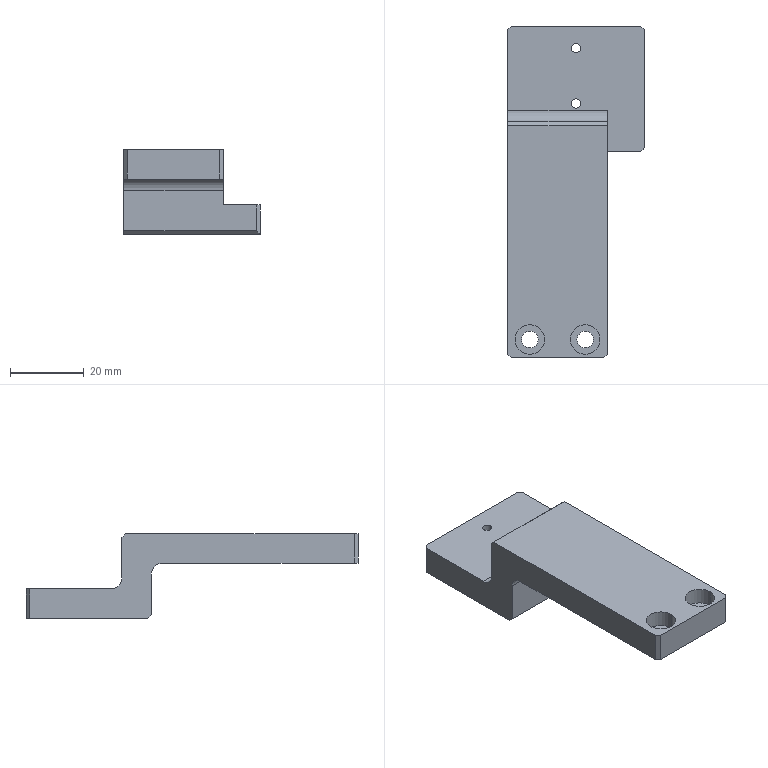Part | SolidWorks | features ICE 3, Chamfer 2, HoleWzd 2, Extrusion 1, Fillet 1 | 1 solid | 34 faces | box 37 x 90 x 23 mm | volume 24810 mm3 | plane 20 | cylinder 14 | commonest cylinder face diameters 2.5 x4 4.5 x4 8 x4 6 x2
STEP:
#1=CARTESIAN_POINT('',(2.,-85.,-0.5));
#2=VERTEX_POINT('',#1);
#3=CARTESIAN_POINT('',(10.,-85.,-0.5));
#4=VERTEX_POINT('',#3);
#5=CARTESIAN_POINT('',(6.,-85.,-0.5));
#6=DIRECTION('',(0.,0.,1.));
#7=DIRECTION('',(1.,0.,0.));
#8=AXIS2_PLACEMENT_3D('',#5,#6,#7);
#9=CIRCLE('',#8,4.);
#10=EDGE_CURVE('',#2,#4,#9,.T.);
#11=ORIENTED_EDGE('',*,*,#10,.F.);
#12=CARTESIAN_POINT('',(2.,-85.,4.));
#13=VERTEX_POINT('',#12);
#14=CARTESIAN_POINT('',(2.,-85.,4.));
#15=DIRECTION('',(0.,0.,1.));
#16=VECTOR('',#15,1000.);
#17=LINE('',#14,#16);
#18=EDGE_CURVE('',#2,#13,#17,.T.);
#19=ORIENTED_EDGE('',*,*,#18,.T.);
#20=CARTESIAN_POINT('',(10.,-85.,4.));
#21=VERTEX_POINT('',#20);
#22=CARTESIAN_POINT('',(6.,-85.,4.));
#23=DIRECTION('',(0.,0.,1.));
#24=DIRECTION('',(1.,0.,0.));
#25=AXIS2_PLACEMENT_3D('',#22,#23,#24);
#26=CIRCLE('',#25,4.);
#27=EDGE_CURVE('',#13,#21,#26,.T.);
#28=ORIENTED_EDGE('',*,*,#27,.T.);
#29=CARTESIAN_POINT('',(10.,-85.,4.));
#30=DIRECTION('',(0.,0.,1.));
#31=VECTOR('',#30,1000.);
#32=LINE('',#29,#31);
#33=EDGE_CURVE('',#4,#21,#32,.T.);
#34=ORIENTED_EDGE('',*,*,#33,.F.);
#35=EDGE_LOOP('',(#11,#19,#28,#34));
#36=FACE_OUTER_BOUND('',#35,.T.);
#37=CARTESIAN_POINT('',(6.,-85.,4.));
#38=DIRECTION('',(0.,0.,1.));
#39=DIRECTION('',(1.,0.,0.));
#40=AXIS2_PLACEMENT_3D('',#37,#38,#39);
#41=CYLINDRICAL_SURFACE('',#40,4.);
#42=ADVANCED_FACE('',(#36),#41,.F.);
#43=CARTESIAN_POINT('',(3.75,-85.,-4.));
#44=VERTEX_POINT('',#43);
#45=CARTESIAN_POINT('',(8.25,-85.,-4.));
#46=VERTEX_POINT('',#45);
#47=CARTESIAN_POINT('',(6.,-85.,-4.));
#48=DIRECTION('',(0.,0.,1.));
#49=DIRECTION('',(1.,0.,0.));
#50=AXIS2_PLACEMENT_3D('',#47,#48,#49);
#51=CIRCLE('',#50,2.25);
#52=EDGE_CURVE('',#44,#46,#51,.T.);
#53=ORIENTED_EDGE('',*,*,#52,.F.);
#54=CARTESIAN_POINT('',(3.75,-85.,-0.5));
#55=VERTEX_POINT('',#54);
#56=CARTESIAN_POINT('',(3.75,-85.,4.));
#57=DIRECTION('',(0.,0.,1.));
#58=VECTOR('',#57,1000.);
#59=LINE('',#56,#58);
#60=EDGE_CURVE('',#44,#55,#59,.T.);
#61=ORIENTED_EDGE('',*,*,#60,.T.);
#62=CARTESIAN_POINT('',(8.25,-85.,-0.5));
#63=VERTEX_POINT('',#62);
#64=CARTESIAN_POINT('',(6.,-85.,-0.5));
#65=DIRECTION('',(0.,0.,1.));
#66=DIRECTION('',(1.,0.,0.));
#67=AXIS2_PLACEMENT_3D('',#64,#65,#66);
#68=CIRCLE('',#67,2.25);
#69=EDGE_CURVE('',#55,#63,#68,.T.);
#70=ORIENTED_EDGE('',*,*,#69,.T.);
#71=CARTESIAN_POINT('',(8.25,-85.,4.));
#72=DIRECTION('',(0.,0.,1.));
#73=VECTOR('',#72,1000.);
#74=LINE('',#71,#73);
#75=EDGE_CURVE('',#46,#63,#74,.T.);
#76=ORIENTED_EDGE('',*,*,#75,.F.);
#77=EDGE_LOOP('',(#53,#61,#70,#76));
#78=FACE_OUTER_BOUND('',#77,.T.);
#79=CARTESIAN_POINT('',(6.,-85.,4.));
#80=DIRECTION('',(0.,0.,1.));
#81=DIRECTION('',(1.,0.,0.));
#82=AXIS2_PLACEMENT_3D('',#79,#80,#81);
#83=CYLINDRICAL_SURFACE('',#82,2.25);
#84=ADVANCED_FACE('',(#78),#83,.F.);
#85=CARTESIAN_POINT('',(17.,-85.,-0.5));
#86=VERTEX_POINT('',#85);
#87=CARTESIAN_POINT('',(25.,-85.,-0.5));
#88=VERTEX_POINT('',#87);
#89=CARTESIAN_POINT('',(21.,-85.,-0.5));
#90=DIRECTION('',(0.,0.,1.));
#91=DIRECTION('',(1.,0.,0.));
#92=AXIS2_PLACEMENT_3D('',#89,#90,#91);
#93=CIRCLE('',#92,4.);
#94=EDGE_CURVE('',#86,#88,#93,.T.);
#95=ORIENTED_EDGE('',*,*,#94,.F.);
#96=CARTESIAN_POINT('',(17.,-85.,4.));
#97=VERTEX_POINT('',#96);
#98=CARTESIAN_POINT('',(17.,-85.,4.));
#99=DIRECTION('',(0.,0.,1.));
#100=VECTOR('',#99,1000.);
#101=LINE('',#98,#100);
#102=EDGE_CURVE('',#86,#97,#101,.T.);
#103=ORIENTED_EDGE('',*,*,#102,.T.);
#104=CARTESIAN_POINT('',(25.,-85.,4.));
#105=VERTEX_POINT('',#104);
#106=CARTESIAN_POINT('',(21.,-85.,4.));
#107=DIRECTION('',(0.,0.,1.));
#108=DIRECTION('',(1.,0.,0.));
#109=AXIS2_PLACEMENT_3D('',#106,#107,#108);
#110=CIRCLE('',#109,4.);
#111=EDGE_CURVE('',#97,#105,#110,.T.);
#112=ORIENTED_EDGE('',*,*,#111,.T.);
#113=CARTESIAN_POINT('',(25.,-85.,4.));
#114=DIRECTION('',(0.,0.,1.));
#115=VECTOR('',#114,1000.);
#116=LINE('',#113,#115);
#117=EDGE_CURVE('',#88,#105,#116,.T.);
#118=ORIENTED_EDGE('',*,*,#117,.F.);
#119=EDGE_LOOP('',(#95,#103,#112,#118));
#120=FACE_OUTER_BOUND('',#119,.T.);
#121=CARTESIAN_POINT('',(21.,-85.,4.));
#122=DIRECTION('',(0.,0.,1.));
#123=DIRECTION('',(1.,0.,0.));
#124=AXIS2_PLACEMENT_3D('',#121,#122,#123);
#125=CYLINDRICAL_SURFACE('',#124,4.);
#126=ADVANCED_FACE('',(#120),#125,.F.);
#127=CARTESIAN_POINT('',(18.75,-85.,-4.));
#128=VERTEX_POINT('',#127);
#129=CARTESIAN_POINT('',(23.25,-85.,-4.));
#130=VERTEX_POINT('',#129);
#131=CARTESIAN_POINT('',(21.,-85.,-4.));
#132=DIRECTION('',(0.,0.,1.));
#133=DIRECTION('',(1.,0.,0.));
#134=AXIS2_PLACEMENT_3D('',#131,#132,#133);
#135=CIRCLE('',#134,2.25);
#136=EDGE_CURVE('',#128,#130,#135,.T.);
#137=ORIENTED_EDGE('',*,*,#136,.F.);
#138=CARTESIAN_POINT('',(18.75,-85.,-0.5));
#139=VERTEX_POINT('',#138);
#140=CARTESIAN_POINT('',(18.75,-85.,4.));
#141=DIRECTION('',(0.,0.,1.));
#142=VECTOR('',#141,1000.);
#143=LINE('',#140,#142);
#144=EDGE_CURVE('',#128,#139,#143,.T.);
#145=ORIENTED_EDGE('',*,*,#144,.T.);
#146=CARTESIAN_POINT('',(23.25,-85.,-0.5));
#147=VERTEX_POINT('',#146);
#148=CARTESIAN_POINT('',(21.,-85.,-0.5));
#149=DIRECTION('',(0.,0.,1.));
#150=DIRECTION('',(1.,0.,0.));
#151=AXIS2_PLACEMENT_3D('',#148,#149,#150);
#152=CIRCLE('',#151,2.25);
#153=EDGE_CURVE('',#139,#147,#152,.T.);
#154=ORIENTED_EDGE('',*,*,#153,.T.);
#155=CARTESIAN_POINT('',(23.25,-85.,4.));
#156=DIRECTION('',(0.,0.,1.));
#157=VECTOR('',#156,1000.);
#158=LINE('',#155,#157);
#159=EDGE_CURVE('',#130,#147,#158,.T.);
#160=ORIENTED_EDGE('',*,*,#159,.F.);
#161=EDGE_LOOP('',(#137,#145,#154,#160));
#162=FACE_OUTER_BOUND('',#161,.T.);
#163=CARTESIAN_POINT('',(21.,-85.,4.));
#164=DIRECTION('',(0.,0.,1.));
#165=DIRECTION('',(1.,0.,0.));
#166=AXIS2_PLACEMENT_3D('',#163,#164,#165);
#167=CYLINDRICAL_SURFACE('',#166,2.25);
#168=ADVANCED_FACE('',(#162),#167,.F.);
#169=CARTESIAN_POINT('',(17.25,-21.,-19.));
#170=VERTEX_POINT('',#169);
#171=CARTESIAN_POINT('',(19.75,-21.,-19.));
#172=VERTEX_POINT('',#171);
#173=CARTESIAN_POINT('',(18.5,-21.,-19.));
#174=DIRECTION('',(0.,0.,1.));
#175=DIRECTION('',(1.,0.,0.));
#176=AXIS2_PLACEMENT_3D('',#173,#174,#175);
#177=CIRCLE('',#176,1.25);
#178=EDGE_CURVE('',#170,#172,#177,.T.);
#179=ORIENTED_EDGE('',*,*,#178,.F.);
#180=CARTESIAN_POINT('',(17.25,-21.,-11.));
#181=VERTEX_POINT('',#180);
#182=CARTESIAN_POINT('',(17.25,-21.,4.));
#183=DIRECTION('',(0.,0.,1.));
#184=VECTOR('',#183,1000.);
#185=LINE('',#182,#184);
#186=EDGE_CURVE('',#170,#181,#185,.T.);
#187=ORIENTED_EDGE('',*,*,#186,.T.);
#188=CARTESIAN_POINT('',(19.75,-21.,-11.));
#189=VERTEX_POINT('',#188);
#190=CARTESIAN_POINT('',(18.5,-21.,-11.));
#191=DIRECTION('',(0.,0.,1.));
#192=DIRECTION('',(0.,1.,0.));
#193=AXIS2_PLACEMENT_3D('',#190,#191,#192);
#194=CIRCLE('',#193,1.25);
#195=EDGE_CURVE('',#181,#189,#194,.T.);
#196=ORIENTED_EDGE('',*,*,#195,.T.);
#197=CARTESIAN_POINT('',(19.75,-21.,4.));
#198=DIRECTION('',(0.,0.,1.));
#199=VECTOR('',#198,1000.);
#200=LINE('',#197,#199);
#201=EDGE_CURVE('',#172,#189,#200,.T.);
#202=ORIENTED_EDGE('',*,*,#201,.F.);
#203=EDGE_LOOP('',(#179,#187,#196,#202));
#204=FACE_OUTER_BOUND('',#203,.T.);
#205=CARTESIAN_POINT('',(18.5,-21.,4.));
#206=DIRECTION('',(0.,0.,1.));
#207=DIRECTION('',(1.,0.,0.));
#208=AXIS2_PLACEMENT_3D('',#205,#206,#207);
#209=CYLINDRICAL_SURFACE('',#208,1.25);
#210=ADVANCED_FACE('',(#204),#209,.F.);
#211=CARTESIAN_POINT('',(17.25,-6.,-19.));
#212=VERTEX_POINT('',#211);
#213=CARTESIAN_POINT('',(19.75,-6.,-19.));
#214=VERTEX_POINT('',#213);
#215=CARTESIAN_POINT('',(18.5,-6.,-19.));
#216=DIRECTION('',(0.,0.,1.));
#217=DIRECTION('',(1.,0.,0.));
#218=AXIS2_PLACEMENT_3D('',#215,#216,#217);
#219=CIRCLE('',#218,1.25);
#220=EDGE_CURVE('',#212,#214,#219,.T.);
#221=ORIENTED_EDGE('',*,*,#220,.F.);
#222=CARTESIAN_POINT('',(17.25,-6.,-11.));
#223=VERTEX_POINT('',#222);
#224=CARTESIAN_POINT('',(17.25,-6.,4.));
#225=DIRECTION('',(0.,0.,1.));
#226=VECTOR('',#225,1000.);
#227=LINE('',#224,#226);
#228=EDGE_CURVE('',#212,#223,#227,.T.);
#229=ORIENTED_EDGE('',*,*,#228,.T.);
#230=CARTESIAN_POINT('',(19.75,-6.,-11.));
#231=VERTEX_POINT('',#230);
#232=CARTESIAN_POINT('',(18.5,-6.,-11.));
#233=DIRECTION('',(0.,0.,1.));
#234=DIRECTION('',(0.,1.,0.));
#235=AXIS2_PLACEMENT_3D('',#232,#233,#234);
#236=CIRCLE('',#235,1.25);
#237=EDGE_CURVE('',#223,#231,#236,.T.);
#238=ORIENTED_EDGE('',*,*,#237,.T.);
#239=CARTESIAN_POINT('',(19.75,-6.,4.));
#240=DIRECTION('',(0.,0.,1.));
#241=VECTOR('',#240,1000.);
#242=LINE('',#239,#241);
#243=EDGE_CURVE('',#214,#231,#242,.T.);
#244=ORIENTED_EDGE('',*,*,#243,.F.);
#245=EDGE_LOOP('',(#221,#229,#238,#244));
#246=FACE_OUTER_BOUND('',#245,.T.);
#247=CARTESIAN_POINT('',(18.5,-6.,4.));
#248=DIRECTION('',(0.,0.,1.));
#249=DIRECTION('',(1.,0.,0.));
#250=AXIS2_PLACEMENT_3D('',#247,#248,#249);
#251=CYLINDRICAL_SURFACE('',#250,1.25);
#252=ADVANCED_FACE('',(#246),#251,.F.);
#253=CARTESIAN_POINT('',(0.,-1.,-19.));
#254=VERTEX_POINT('',#253);
#255=CARTESIAN_POINT('',(0.,-33.,-19.));
#256=VERTEX_POINT('',#255);
#257=CARTESIAN_POINT('',(0.,0.,-19.));
#258=DIRECTION('',(0.,-1.,0.));
#259=VECTOR('',#258,1000.);
#260=LINE('',#257,#259);
#261=EDGE_CURVE('',#254,#256,#260,.T.);
#262=ORIENTED_EDGE('',*,*,#261,.T.);
#263=CARTESIAN_POINT('',(0.,-34.,-18.));
#264=VERTEX_POINT('',#263);
#265=CARTESIAN_POINT('',(0.,-34.,-18.));
#266=DIRECTION('',(0.,-0.7071,0.7071));
#267=VECTOR('',#266,1000.);
#268=LINE('',#265,#267);
#269=EDGE_CURVE('',#256,#264,#268,.T.);
#270=ORIENTED_EDGE('',*,*,#269,.T.);
#271=CARTESIAN_POINT('',(0.,-34.,-7.));
#272=VERTEX_POINT('',#271);
#273=CARTESIAN_POINT('',(0.,-34.,-19.));
#274=DIRECTION('',(0.,0.,1.));
#275=VECTOR('',#274,1000.);
#276=LINE('',#273,#275);
#277=EDGE_CURVE('',#264,#272,#276,.T.);
#278=ORIENTED_EDGE('',*,*,#277,.T.);
#279=CARTESIAN_POINT('',(0.,-37.,-4.));
#280=VERTEX_POINT('',#279);
#281=CARTESIAN_POINT('',(0.,-37.,-7.));
#282=DIRECTION('',(1.,0.,0.));
#283=DIRECTION('',(0.,1.,0.));
#284=AXIS2_PLACEMENT_3D('',#281,#282,#283);
#285=CIRCLE('',#284,3.);
#286=EDGE_CURVE('',#272,#280,#285,.T.);
#287=ORIENTED_EDGE('',*,*,#286,.T.);
#288=CARTESIAN_POINT('',(0.,-89.,-4.));
#289=VERTEX_POINT('',#288);
#290=CARTESIAN_POINT('',(0.,0.,-4.));
#291=DIRECTION('',(0.,-1.,0.));
#292=VECTOR('',#291,1000.);
#293=LINE('',#290,#292);
#294=EDGE_CURVE('',#280,#289,#293,.T.);
#295=ORIENTED_EDGE('',*,*,#294,.T.);
#296=CARTESIAN_POINT('',(0.,-89.,4.));
#297=VERTEX_POINT('',#296);
#298=CARTESIAN_POINT('',(0.,-89.,4.));
#299=DIRECTION('',(0.,0.,1.));
#300=VECTOR('',#299,1000.);
#301=LINE('',#298,#300);
#302=EDGE_CURVE('',#289,#297,#301,.T.);
#303=ORIENTED_EDGE('',*,*,#302,.T.);
#304=CARTESIAN_POINT('',(0.,-27.,4.));
#305=VERTEX_POINT('',#304);
#306=CARTESIAN_POINT('',(0.,0.,4.));
#307=DIRECTION('',(0.,-1.,0.));
#308=VECTOR('',#307,1000.);
#309=LINE('',#306,#308);
#310=EDGE_CURVE('',#305,#297,#309,.T.);
#311=ORIENTED_EDGE('',*,*,#310,.F.);
#312=CARTESIAN_POINT('',(0.,-26.,3.));
#313=VERTEX_POINT('',#312);
#314=CARTESIAN_POINT('',(0.,-26.,3.));
#315=DIRECTION('',(0.,0.7071,-0.7071));
#316=VECTOR('',#315,1000.);
#317=LINE('',#314,#316);
#318=EDGE_CURVE('',#305,#313,#317,.T.);
#319=ORIENTED_EDGE('',*,*,#318,.T.);
#320=CARTESIAN_POINT('',(0.,-26.,-8.));
#321=VERTEX_POINT('',#320);
#322=CARTESIAN_POINT('',(0.,-26.,4.));
#323=DIRECTION('',(0.,0.,-1.));
#324=VECTOR('',#323,1000.);
#325=LINE('',#322,#324);
#326=EDGE_CURVE('',#313,#321,#325,.T.);
#327=ORIENTED_EDGE('',*,*,#326,.T.);
#328=CARTESIAN_POINT('',(0.,-23.,-11.));
#329=VERTEX_POINT('',#328);
#330=CARTESIAN_POINT('',(0.,-23.,-8.));
#331=DIRECTION('',(1.,0.,0.));
#332=DIRECTION('',(0.,1.,0.));
#333=AXIS2_PLACEMENT_3D('',#330,#331,#332);
#334=CIRCLE('',#333,3.);
#335=EDGE_CURVE('',#321,#329,#334,.T.);
#336=ORIENTED_EDGE('',*,*,#335,.T.);
#337=CARTESIAN_POINT('',(0.,-1.,-11.));
#338=VERTEX_POINT('',#337);
#339=CARTESIAN_POINT('',(0.,0.,-11.));
#340=DIRECTION('',(0.,1.,0.));
#341=VECTOR('',#340,1000.);
#342=LINE('',#339,#341);
#343=EDGE_CURVE('',#329,#338,#342,.T.);
#344=ORIENTED_EDGE('',*,*,#343,.T.);
#345=CARTESIAN_POINT('',(0.,-1.,4.));
#346=DIRECTION('',(0.,0.,-1.));
#347=VECTOR('',#346,1000.);
#348=LINE('',#345,#347);
#349=EDGE_CURVE('',#338,#254,#348,.T.);
#350=ORIENTED_EDGE('',*,*,#349,.T.);
#351=EDGE_LOOP('',(#262,#270,#278,#287,#295,#303,#311,#319,#327,#336,#344,#350));
#352=FACE_OUTER_BOUND('',#351,.T.);
#353=CARTESIAN_POINT('',(0.,0.,4.));
#354=DIRECTION('',(1.,0.,0.));
#355=DIRECTION('',(0.,1.,0.));
#356=AXIS2_PLACEMENT_3D('',#353,#354,#355);
#357=PLANE('',#356);
#358=ADVANCED_FACE('',(#352),#357,.F.);
#359=CARTESIAN_POINT('',(1.,-90.,4.));
#360=VERTEX_POINT('',#359);
#361=CARTESIAN_POINT('',(26.,-90.,4.));
#362=VERTEX_POINT('',#361);
#363=CARTESIAN_POINT('',(0.,-90.,4.));
#364=DIRECTION('',(1.,0.,0.));
#365=VECTOR('',#364,1000.);
#366=LINE('',#363,#365);
#367=EDGE_CURVE('',#360,#362,#366,.T.);
#368=ORIENTED_EDGE('',*,*,#367,.F.);
#369=CARTESIAN_POINT('',(1.,-90.,-4.));
#370=VERTEX_POINT('',#369);
#371=CARTESIAN_POINT('',(1.,-90.,4.));
#372=DIRECTION('',(0.,0.,-1.));
#373=VECTOR('',#372,1000.);
#374=LINE('',#371,#373);
#375=EDGE_CURVE('',#360,#370,#374,.T.);
#376=ORIENTED_EDGE('',*,*,#375,.T.);
#377=CARTESIAN_POINT('',(26.,-90.,-4.));
#378=VERTEX_POINT('',#377);
#379=CARTESIAN_POINT('',(0.,-90.,-4.));
#380=DIRECTION('',(1.,0.,0.));
#381=VECTOR('',#380,1000.);
#382=LINE('',#379,#381);
#383=EDGE_CURVE('',#370,#378,#382,.T.);
#384=ORIENTED_EDGE('',*,*,#383,.T.);
#385=CARTESIAN_POINT('',(26.,-90.,4.));
#386=DIRECTION('',(0.,0.,1.));
#387=VECTOR('',#386,1000.);
#388=LINE('',#385,#387);
#389=EDGE_CURVE('',#378,#362,#388,.T.);
#390=ORIENTED_EDGE('',*,*,#389,.T.);
#391=EDGE_LOOP('',(#368,#376,#384,#390));
#392=FACE_OUTER_BOUND('',#391,.T.);
#393=CARTESIAN_POINT('',(0.,-90.,4.));
#394=DIRECTION('',(0.,1.,0.));
#395=DIRECTION('',(0.,0.,1.));
#396=AXIS2_PLACEMENT_3D('',#393,#394,#395);
#397=PLANE('',#396);
#398=ADVANCED_FACE('',(#392),#397,.F.);
#399=CARTESIAN_POINT('',(37.,-33.,-11.));
#400=VERTEX_POINT('',#399);
#401=CARTESIAN_POINT('',(37.,-1.,-11.));
#402=VERTEX_POINT('',#401);
#403=CARTESIAN_POINT('',(37.,0.,-11.));
#404=DIRECTION('',(0.,1.,0.));
#405=VECTOR('',#404,1000.);
#406=LINE('',#403,#405);
#407=EDGE_CURVE('',#400,#402,#406,.T.);
#408=ORIENTED_EDGE('',*,*,#407,.F.);
#409=CARTESIAN_POINT('',(37.,-33.,-19.));
#410=VERTEX_POINT('',#409);
#411=CARTESIAN_POINT('',(37.,-33.,-19.));
#412=DIRECTION('',(0.,0.,-1.));
#413=VECTOR('',#412,1000.);
#414=LINE('',#411,#413);
#415=EDGE_CURVE('',#400,#410,#414,.T.);
#416=ORIENTED_EDGE('',*,*,#415,.T.);
#417=CARTESIAN_POINT('',(37.,-1.,-19.));
#418=VERTEX_POINT('',#417);
#419=CARTESIAN_POINT('',(37.,0.,-19.));
#420=DIRECTION('',(0.,1.,0.));
#421=VECTOR('',#420,1000.);
#422=LINE('',#419,#421);
#423=EDGE_CURVE('',#410,#418,#422,.T.);
#424=ORIENTED_EDGE('',*,*,#423,.T.);
#425=CARTESIAN_POINT('',(37.,-1.,4.));
#426=DIRECTION('',(0.,0.,1.));
#427=VECTOR('',#426,1000.);
#428=LINE('',#425,#427);
#429=EDGE_CURVE('',#418,#402,#428,.T.);
#430=ORIENTED_EDGE('',*,*,#429,.T.);
#431=EDGE_LOOP('',(#408,#416,#424,#430));
#432=FACE_OUTER_BOUND('',#431,.T.);
#433=CARTESIAN_POINT('',(37.,0.,4.));
#434=DIRECTION('',(-1.,0.,0.));
#435=DIRECTION('',(0.,-1.,0.));
#436=AXIS2_PLACEMENT_3D('',#433,#434,#435);
#437=PLANE('',#436);
#438=ADVANCED_FACE('',(#432),#437,.F.);
#439=CARTESIAN_POINT('',(1.,0.,-11.));
#440=VERTEX_POINT('',#439);
#441=CARTESIAN_POINT('',(36.,0.,-11.));
#442=VERTEX_POINT('',#441);
#443=CARTESIAN_POINT('',(-0.00005,0.,-11.));
#444=DIRECTION('',(1.,0.,0.));
#445=VECTOR('',#444,1000.);
#446=LINE('',#443,#445);
#447=EDGE_CURVE('',#440,#442,#446,.T.);
#448=ORIENTED_EDGE('',*,*,#447,.T.);
#449=CARTESIAN_POINT('',(36.,0.,-19.));
#450=VERTEX_POINT('',#449);
#451=CARTESIAN_POINT('',(36.,0.,4.));
#452=DIRECTION('',(0.,0.,-1.));
#453=VECTOR('',#452,1000.);
#454=LINE('',#451,#453);
#455=EDGE_CURVE('',#442,#450,#454,.T.);
#456=ORIENTED_EDGE('',*,*,#455,.T.);
#457=CARTESIAN_POINT('',(1.,0.,-19.));
#458=VERTEX_POINT('',#457);
#459=CARTESIAN_POINT('',(0.,0.,-19.));
#460=DIRECTION('',(-1.,0.,0.));
#461=VECTOR('',#460,1000.);
#462=LINE('',#459,#461);
#463=EDGE_CURVE('',#450,#458,#462,.T.);
#464=ORIENTED_EDGE('',*,*,#463,.T.);
#465=CARTESIAN_POINT('',(1.,0.,4.));
#466=DIRECTION('',(0.,0.,1.));
#467=VECTOR('',#466,1000.);
#468=LINE('',#465,#467);
#469=EDGE_CURVE('',#458,#440,#468,.T.);
#470=ORIENTED_EDGE('',*,*,#469,.T.);
#471=EDGE_LOOP('',(#448,#456,#464,#470));
#472=FACE_OUTER_BOUND('',#471,.T.);
#473=CARTESIAN_POINT('',(0.,0.,4.));
#474=DIRECTION('',(0.,-1.,0.));
#475=DIRECTION('',(0.,0.,-1.));
#476=AXIS2_PLACEMENT_3D('',#473,#474,#475);
#477=PLANE('',#476);
#478=ADVANCED_FACE('',(#472),#477,.F.);
#479=CARTESIAN_POINT('',(27.,-27.,4.));
#480=VERTEX_POINT('',#479);
#481=CARTESIAN_POINT('',(27.,-89.,4.));
#482=VERTEX_POINT('',#481);
#483=CARTESIAN_POINT('',(27.,-90.,4.));
#484=DIRECTION('',(0.,-1.,0.));
#485=VECTOR('',#484,1000.);
#486=LINE('',#483,#485);
#487=EDGE_CURVE('',#480,#482,#486,.T.);
#488=ORIENTED_EDGE('',*,*,#487,.F.);
#489=CARTESIAN_POINT('',(0.,-27.,4.));
#490=DIRECTION('',(-1.,0.,0.));
#491=VECTOR('',#490,1000.);
#492=LINE('',#489,#491);
#493=EDGE_CURVE('',#480,#305,#492,.T.);
#494=ORIENTED_EDGE('',*,*,#493,.T.);
#495=ORIENTED_EDGE('',*,*,#310,.T.);
#496=CARTESIAN_POINT('',(0.5,-89.5,4.));
#497=DIRECTION('',(0.7071,-0.7071,0.));
#498=VECTOR('',#497,1000.);
#499=LINE('',#496,#498);
#500=EDGE_CURVE('',#297,#360,#499,.T.);
#501=ORIENTED_EDGE('',*,*,#500,.T.);
#502=ORIENTED_EDGE('',*,*,#367,.T.);
#503=CARTESIAN_POINT('',(13.,-103.,4.));
#504=DIRECTION('',(0.7071,0.7071,0.));
#505=VECTOR('',#504,1000.);
#506=LINE('',#503,#505);
#507=EDGE_CURVE('',#362,#482,#506,.T.);
#508=ORIENTED_EDGE('',*,*,#507,.T.);
#509=EDGE_LOOP('',(#488,#494,#495,#501,#502,#508));
#510=FACE_OUTER_BOUND('',#509,.T.);
#511=CARTESIAN_POINT('',(6.,-85.,4.));
#512=DIRECTION('',(0.,0.,1.));
#513=DIRECTION('',(1.,0.,0.));
#514=AXIS2_PLACEMENT_3D('',#511,#512,#513);
#515=CIRCLE('',#514,4.);
#516=EDGE_CURVE('',#21,#13,#515,.T.);
#517=ORIENTED_EDGE('',*,*,#516,.F.);
#518=ORIENTED_EDGE('',*,*,#27,.F.);
#519=EDGE_LOOP('',(#517,#518));
#520=FACE_BOUND('',#519,.T.);
#521=CARTESIAN_POINT('',(21.,-85.,4.));
#522=DIRECTION('',(0.,0.,1.));
#523=DIRECTION('',(1.,0.,0.));
#524=AXIS2_PLACEMENT_3D('',#521,#522,#523);
#525=CIRCLE('',#524,4.);
#526=EDGE_CURVE('',#105,#97,#525,.T.);
#527=ORIENTED_EDGE('',*,*,#526,.F.);
#528=ORIENTED_EDGE('',*,*,#111,.F.);
#529=EDGE_LOOP('',(#527,#528));
#530=FACE_BOUND('',#529,.T.);
#531=CARTESIAN_POINT('',(0.,-90.,4.));
#532=DIRECTION('',(0.,0.,1.));
#533=DIRECTION('',(1.,0.,0.));
#534=AXIS2_PLACEMENT_3D('',#531,#532,#533);
#535=PLANE('',#534);
#536=ADVANCED_FACE('',(#510,#520,#530),#535,.T.);
#537=CARTESIAN_POINT('',(6.,-85.,-4.));
#538=DIRECTION('',(0.,0.,1.));
#539=DIRECTION('',(1.,0.,0.));
#540=AXIS2_PLACEMENT_3D('',#537,#538,#539);
#541=CIRCLE('',#540,2.25);
#542=EDGE_CURVE('',#46,#44,#541,.T.);
#543=ORIENTED_EDGE('',*,*,#542,.T.);
#544=ORIENTED_EDGE('',*,*,#52,.T.);
#545=EDGE_LOOP('',(#543,#544));
#546=FACE_BOUND('',#545,.T.);
#547=CARTESIAN_POINT('',(21.,-85.,-4.));
#548=DIRECTION('',(0.,0.,1.));
#549=DIRECTION('',(1.,0.,0.));
#550=AXIS2_PLACEMENT_3D('',#547,#548,#549);
#551=CIRCLE('',#550,2.25);
#552=EDGE_CURVE('',#130,#128,#551,.T.);
#553=ORIENTED_EDGE('',*,*,#552,.T.);
#554=ORIENTED_EDGE('',*,*,#136,.T.);
#555=EDGE_LOOP('',(#553,#554));
#556=FACE_BOUND('',#555,.T.);
#557=ORIENTED_EDGE('',*,*,#383,.F.);
#558=CARTESIAN_POINT('',(1.,-90.,-4.));
#559=DIRECTION('',(-0.7071,0.7071,0.));
#560=VECTOR('',#559,1000.);
#561=LINE('',#558,#560);
#562=EDGE_CURVE('',#370,#289,#561,.T.);
#563=ORIENTED_EDGE('',*,*,#562,.T.);
#564=ORIENTED_EDGE('',*,*,#294,.F.);
#565=CARTESIAN_POINT('',(27.,-37.,-4.));
#566=VERTEX_POINT('',#565);
#567=CARTESIAN_POINT('',(0.,-37.,-4.));
#568=DIRECTION('',(1.,0.,0.));
#569=VECTOR('',#568,1000.);
#570=LINE('',#567,#569);
#571=EDGE_CURVE('',#280,#566,#570,.T.);
#572=ORIENTED_EDGE('',*,*,#571,.T.);
#573=CARTESIAN_POINT('',(27.,-89.,-4.));
#574=VERTEX_POINT('',#573);
#575=CARTESIAN_POINT('',(27.,-90.,-4.));
#576=DIRECTION('',(0.,-1.,0.));
#577=VECTOR('',#576,1000.);
#578=LINE('',#575,#577);
#579=EDGE_CURVE('',#566,#574,#578,.T.);
#580=ORIENTED_EDGE('',*,*,#579,.T.);
#581=CARTESIAN_POINT('',(26.,-90.,-4.));
#582=DIRECTION('',(-0.7071,-0.7071,0.));
#583=VECTOR('',#582,1000.);
#584=LINE('',#581,#583);
#585=EDGE_CURVE('',#574,#378,#584,.T.);
#586=ORIENTED_EDGE('',*,*,#585,.T.);
#587=EDGE_LOOP('',(#557,#563,#564,#572,#580,#586));
#588=FACE_OUTER_BOUND('',#587,.T.);
#589=CARTESIAN_POINT('',(0.,-90.,-4.));
#590=DIRECTION('',(0.,0.,1.));
#591=DIRECTION('',(1.,0.,0.));
#592=AXIS2_PLACEMENT_3D('',#589,#590,#591);
#593=PLANE('',#592);
#594=ADVANCED_FACE('',(#546,#556,#588),#593,.F.);
#595=ORIENTED_EDGE('',*,*,#277,.F.);
#596=CARTESIAN_POINT('',(36.,-34.,-18.));
#597=VERTEX_POINT('',#596);
#598=CARTESIAN_POINT('',(36.,-34.,-18.));
#599=DIRECTION('',(1.,0.,0.));
#600=VECTOR('',#599,1000.);
#601=LINE('',#598,#600);
#602=EDGE_CURVE('',#264,#597,#601,.T.);
#603=ORIENTED_EDGE('',*,*,#602,.T.);
#604=CARTESIAN_POINT('',(36.,-34.,-11.));
#605=VERTEX_POINT('',#604);
#606=CARTESIAN_POINT('',(36.,-34.,-11.));
#607=DIRECTION('',(0.,0.,1.));
#608=VECTOR('',#607,1000.);
#609=LINE('',#606,#608);
#610=EDGE_CURVE('',#597,#605,#609,.T.);
#611=ORIENTED_EDGE('',*,*,#610,.T.);
#612=CARTESIAN_POINT('',(27.,-34.,-11.));
#613=VERTEX_POINT('',#612);
#614=CARTESIAN_POINT('',(0.,-34.,-11.));
#615=DIRECTION('',(1.,0.,0.));
#616=VECTOR('',#615,1000.);
#617=LINE('',#614,#616);
#618=EDGE_CURVE('',#613,#605,#617,.T.);
#619=ORIENTED_EDGE('',*,*,#618,.F.);
#620=CARTESIAN_POINT('',(27.,-34.,-7.));
#621=VERTEX_POINT('',#620);
#622=CARTESIAN_POINT('',(27.,-34.,-19.));
#623=DIRECTION('',(0.,0.,-1.));
#624=VECTOR('',#623,1000.);
#625=LINE('',#622,#624);
#626=EDGE_CURVE('',#621,#613,#625,.T.);
#627=ORIENTED_EDGE('',*,*,#626,.F.);
#628=CARTESIAN_POINT('',(0.,-34.,-7.));
#629=DIRECTION('',(-1.,0.,0.));
#630=VECTOR('',#629,1000.);
#631=LINE('',#628,#630);
#632=EDGE_CURVE('',#621,#272,#631,.T.);
#633=ORIENTED_EDGE('',*,*,#632,.T.);
#634=EDGE_LOOP('',(#595,#603,#611,#619,#627,#633));
#635=FACE_OUTER_BOUND('',#634,.T.);
#636=CARTESIAN_POINT('',(0.,-34.,-19.));
#637=DIRECTION('',(0.,-1.,0.));
#638=DIRECTION('',(0.,0.,-1.));
#639=AXIS2_PLACEMENT_3D('',#636,#637,#638);
#640=PLANE('',#639);
#641=ADVANCED_FACE('',(#635),#640,.T.);
#642=CARTESIAN_POINT('',(18.5,-21.,-19.));
#643=DIRECTION('',(0.,0.,1.));
#644=DIRECTION('',(1.,0.,0.));
#645=AXIS2_PLACEMENT_3D('',#642,#643,#644);
#646=CIRCLE('',#645,1.25);
#647=EDGE_CURVE('',#172,#170,#646,.T.);
#648=ORIENTED_EDGE('',*,*,#647,.T.);
#649=ORIENTED_EDGE('',*,*,#178,.T.);
#650=EDGE_LOOP('',(#648,#649));
#651=FACE_BOUND('',#650,.T.);
#652=CARTESIAN_POINT('',(18.5,-6.,-19.));
#653=DIRECTION('',(0.,0.,1.));
#654=DIRECTION('',(1.,0.,0.));
#655=AXIS2_PLACEMENT_3D('',#652,#653,#654);
#656=CIRCLE('',#655,1.25);
#657=EDGE_CURVE('',#214,#212,#656,.T.);
#658=ORIENTED_EDGE('',*,*,#657,.T.);
#659=ORIENTED_EDGE('',*,*,#220,.T.);
#660=EDGE_LOOP('',(#658,#659));
#661=FACE_BOUND('',#660,.T.);
#662=ORIENTED_EDGE('',*,*,#423,.F.);
#663=CARTESIAN_POINT('',(0.,-33.,-19.));
#664=DIRECTION('',(-1.,0.,0.));
#665=VECTOR('',#664,1000.);
#666=LINE('',#663,#665);
#667=EDGE_CURVE('',#410,#256,#666,.T.);
#668=ORIENTED_EDGE('',*,*,#667,.T.);
#669=ORIENTED_EDGE('',*,*,#261,.F.);
#670=CARTESIAN_POINT('',(0.,-1.,-19.));
#671=DIRECTION('',(0.7071,0.7071,0.));
#672=VECTOR('',#671,1000.);
#673=LINE('',#670,#672);
#674=EDGE_CURVE('',#254,#458,#673,.T.);
#675=ORIENTED_EDGE('',*,*,#674,.T.);
#676=ORIENTED_EDGE('',*,*,#463,.F.);
#677=CARTESIAN_POINT('',(36.,0.,-19.));
#678=DIRECTION('',(0.7071,-0.7071,0.));
#679=VECTOR('',#678,1000.);
#680=LINE('',#677,#679);
#681=EDGE_CURVE('',#450,#418,#680,.T.);
#682=ORIENTED_EDGE('',*,*,#681,.T.);
#683=EDGE_LOOP('',(#662,#668,#669,#675,#676,#682));
#684=FACE_OUTER_BOUND('',#683,.T.);
#685=CARTESIAN_POINT('',(0.,-34.,-19.));
#686=DIRECTION('',(0.,0.,1.));
#687=DIRECTION('',(1.,0.,0.));
#688=AXIS2_PLACEMENT_3D('',#685,#686,#687);
#689=PLANE('',#688);
#690=ADVANCED_FACE('',(#651,#661,#684),#689,.F.);
#691=ORIENTED_EDGE('',*,*,#228,.F.);
#692=ORIENTED_EDGE('',*,*,#657,.F.);
#693=ORIENTED_EDGE('',*,*,#243,.T.);
#694=CARTESIAN_POINT('',(18.5,-6.,-11.));
#695=DIRECTION('',(0.,0.,1.));
#696=DIRECTION('',(0.,1.,0.));
#697=AXIS2_PLACEMENT_3D('',#694,#695,#696);
#698=CIRCLE('',#697,1.25);
#699=EDGE_CURVE('',#231,#223,#698,.T.);
#700=ORIENTED_EDGE('',*,*,#699,.T.);
#701=EDGE_LOOP('',(#691,#692,#693,#700));
#702=FACE_OUTER_BOUND('',#701,.T.);
#703=CARTESIAN_POINT('',(18.5,-6.,4.));
#704=DIRECTION('',(0.,0.,1.));
#705=DIRECTION('',(1.,0.,0.));
#706=AXIS2_PLACEMENT_3D('',#703,#704,#705);
#707=CYLINDRICAL_SURFACE('',#706,1.25);
#708=ADVANCED_FACE('',(#702),#707,.F.);
#709=ORIENTED_EDGE('',*,*,#186,.F.);
#710=ORIENTED_EDGE('',*,*,#647,.F.);
#711=ORIENTED_EDGE('',*,*,#201,.T.);
#712=CARTESIAN_POINT('',(18.5,-21.,-11.));
#713=DIRECTION('',(0.,0.,1.));
#714=DIRECTION('',(0.,1.,0.));
#715=AXIS2_PLACEMENT_3D('',#712,#713,#714);
#716=CIRCLE('',#715,1.25);
#717=EDGE_CURVE('',#189,#181,#716,.T.);
#718=ORIENTED_EDGE('',*,*,#717,.T.);
#719=EDGE_LOOP('',(#709,#710,#711,#718));
#720=FACE_OUTER_BOUND('',#719,.T.);
#721=CARTESIAN_POINT('',(18.5,-21.,4.));
#722=DIRECTION('',(0.,0.,1.));
#723=DIRECTION('',(1.,0.,0.));
#724=AXIS2_PLACEMENT_3D('',#721,#722,#723);
#725=CYLINDRICAL_SURFACE('',#724,1.25);
#726=ADVANCED_FACE('',(#720),#725,.F.);
#727=ORIENTED_EDGE('',*,*,#144,.F.);
#728=ORIENTED_EDGE('',*,*,#552,.F.);
#729=ORIENTED_EDGE('',*,*,#159,.T.);
#730=CARTESIAN_POINT('',(21.,-85.,-0.5));
#731=DIRECTION('',(0.,0.,1.));
#732=DIRECTION('',(1.,0.,0.));
#733=AXIS2_PLACEMENT_3D('',#730,#731,#732);
#734=CIRCLE('',#733,2.25);
#735=EDGE_CURVE('',#147,#139,#734,.T.);
#736=ORIENTED_EDGE('',*,*,#735,.T.);
#737=EDGE_LOOP('',(#727,#728,#729,#736));
#738=FACE_OUTER_BOUND('',#737,.T.);
#739=CARTESIAN_POINT('',(21.,-85.,4.));
#740=DIRECTION('',(0.,0.,1.));
#741=DIRECTION('',(1.,0.,0.));
#742=AXIS2_PLACEMENT_3D('',#739,#740,#741);
#743=CYLINDRICAL_SURFACE('',#742,2.25);
#744=ADVANCED_FACE('',(#738),#743,.F.);
#745=ORIENTED_EDGE('',*,*,#735,.F.);
#746=ORIENTED_EDGE('',*,*,#153,.F.);
#747=EDGE_LOOP('',(#745,#746));
#748=FACE_BOUND('',#747,.T.);
#749=CARTESIAN_POINT('',(21.,-85.,-0.5));
#750=DIRECTION('',(0.,0.,1.));
#751=DIRECTION('',(1.,0.,0.));
#752=AXIS2_PLACEMENT_3D('',#749,#750,#751);
#753=CIRCLE('',#752,4.);
#754=EDGE_CURVE('',#88,#86,#753,.T.);
#755=ORIENTED_EDGE('',*,*,#754,.T.);
#756=ORIENTED_EDGE('',*,*,#94,.T.);
#757=EDGE_LOOP('',(#755,#756));
#758=FACE_OUTER_BOUND('',#757,.T.);
#759=CARTESIAN_POINT('',(23.25,-85.,-0.5));
#760=DIRECTION('',(0.,0.,-1.));
#761=DIRECTION('',(-1.,0.,0.));
#762=AXIS2_PLACEMENT_3D('',#759,#760,#761);
#763=PLANE('',#762);
#764=ADVANCED_FACE('',(#748,#758),#763,.F.);
#765=ORIENTED_EDGE('',*,*,#102,.F.);
#766=ORIENTED_EDGE('',*,*,#754,.F.);
#767=ORIENTED_EDGE('',*,*,#117,.T.);
#768=ORIENTED_EDGE('',*,*,#526,.T.);
#769=EDGE_LOOP('',(#765,#766,#767,#768));
#770=FACE_OUTER_BOUND('',#769,.T.);
#771=CARTESIAN_POINT('',(21.,-85.,4.));
#772=DIRECTION('',(0.,0.,1.));
#773=DIRECTION('',(1.,0.,0.));
#774=AXIS2_PLACEMENT_3D('',#771,#772,#773);
#775=CYLINDRICAL_SURFACE('',#774,4.);
#776=ADVANCED_FACE('',(#770),#775,.F.);
#777=ORIENTED_EDGE('',*,*,#60,.F.);
#778=ORIENTED_EDGE('',*,*,#542,.F.);
#779=ORIENTED_EDGE('',*,*,#75,.T.);
#780=CARTESIAN_POINT('',(6.,-85.,-0.5));
#781=DIRECTION('',(0.,0.,1.));
#782=DIRECTION('',(1.,0.,0.));
#783=AXIS2_PLACEMENT_3D('',#780,#781,#782);
#784=CIRCLE('',#783,2.25);
#785=EDGE_CURVE('',#63,#55,#784,.T.);
#786=ORIENTED_EDGE('',*,*,#785,.T.);
#787=EDGE_LOOP('',(#777,#778,#779,#786));
#788=FACE_OUTER_BOUND('',#787,.T.);
#789=CARTESIAN_POINT('',(6.,-85.,4.));
#790=DIRECTION('',(0.,0.,1.));
#791=DIRECTION('',(1.,0.,0.));
#792=AXIS2_PLACEMENT_3D('',#789,#790,#791);
#793=CYLINDRICAL_SURFACE('',#792,2.25);
#794=ADVANCED_FACE('',(#788),#793,.F.);
#795=ORIENTED_EDGE('',*,*,#785,.F.);
#796=ORIENTED_EDGE('',*,*,#69,.F.);
#797=EDGE_LOOP('',(#795,#796));
#798=FACE_BOUND('',#797,.T.);
#799=CARTESIAN_POINT('',(6.,-85.,-0.5));
#800=DIRECTION('',(0.,0.,1.));
#801=DIRECTION('',(1.,0.,0.));
#802=AXIS2_PLACEMENT_3D('',#799,#800,#801);
#803=CIRCLE('',#802,4.);
#804=EDGE_CURVE('',#4,#2,#803,.T.);
#805=ORIENTED_EDGE('',*,*,#804,.T.);
#806=ORIENTED_EDGE('',*,*,#10,.T.);
#807=EDGE_LOOP('',(#805,#806));
#808=FACE_OUTER_BOUND('',#807,.T.);
#809=CARTESIAN_POINT('',(8.25,-85.,-0.5));
#810=DIRECTION('',(0.,0.,-1.));
#811=DIRECTION('',(-1.,0.,0.));
#812=AXIS2_PLACEMENT_3D('',#809,#810,#811);
#813=PLANE('',#812);
#814=ADVANCED_FACE('',(#798,#808),#813,.F.);
#815=ORIENTED_EDGE('',*,*,#18,.F.);
#816=ORIENTED_EDGE('',*,*,#804,.F.);
#817=ORIENTED_EDGE('',*,*,#33,.T.);
#818=ORIENTED_EDGE('',*,*,#516,.T.);
#819=EDGE_LOOP('',(#815,#816,#817,#818));
#820=FACE_OUTER_BOUND('',#819,.T.);
#821=CARTESIAN_POINT('',(6.,-85.,4.));
#822=DIRECTION('',(0.,0.,1.));
#823=DIRECTION('',(1.,0.,0.));
#824=AXIS2_PLACEMENT_3D('',#821,#822,#823);
#825=CYLINDRICAL_SURFACE('',#824,4.);
#826=ADVANCED_FACE('',(#820),#825,.F.);
#827=ORIENTED_EDGE('',*,*,#326,.F.);
#828=CARTESIAN_POINT('',(27.,-26.,3.));
#829=VERTEX_POINT('',#828);
#830=CARTESIAN_POINT('',(27.,-26.,3.));
#831=DIRECTION('',(1.,0.,0.));
#832=VECTOR('',#831,1000.);
#833=LINE('',#830,#832);
#834=EDGE_CURVE('',#313,#829,#833,.T.);
#835=ORIENTED_EDGE('',*,*,#834,.T.);
#836=CARTESIAN_POINT('',(27.,-26.,-8.));
#837=VERTEX_POINT('',#836);
#838=CARTESIAN_POINT('',(27.,-26.,-75.777));
#839=DIRECTION('',(0.,0.,1.));
#840=VECTOR('',#839,1000.);
#841=LINE('',#838,#840);
#842=EDGE_CURVE('',#837,#829,#841,.T.);
#843=ORIENTED_EDGE('',*,*,#842,.F.);
#844=CARTESIAN_POINT('',(0.,-26.,-8.));
#845=DIRECTION('',(-1.,0.,0.));
#846=VECTOR('',#845,1000.);
#847=LINE('',#844,#846);
#848=EDGE_CURVE('',#837,#321,#847,.T.);
#849=ORIENTED_EDGE('',*,*,#848,.T.);
#850=EDGE_LOOP('',(#827,#835,#843,#849));
#851=FACE_OUTER_BOUND('',#850,.T.);
#852=CARTESIAN_POINT('',(-0.00005,-26.,4.));
#853=DIRECTION('',(0.,-1.,0.));
#854=DIRECTION('',(1.,0.,0.));
#855=AXIS2_PLACEMENT_3D('',#852,#853,#854);
#856=PLANE('',#855);
#857=ADVANCED_FACE('',(#851),#856,.F.);
#858=ORIENTED_EDGE('',*,*,#699,.F.);
#859=ORIENTED_EDGE('',*,*,#237,.F.);
#860=EDGE_LOOP('',(#858,#859));
#861=FACE_BOUND('',#860,.T.);
#862=ORIENTED_EDGE('',*,*,#717,.F.);
#863=ORIENTED_EDGE('',*,*,#195,.F.);
#864=EDGE_LOOP('',(#862,#863));
#865=FACE_BOUND('',#864,.T.);
#866=ORIENTED_EDGE('',*,*,#618,.T.);
#867=CARTESIAN_POINT('',(36.,-34.,-11.));
#868=DIRECTION('',(0.7071,0.7071,0.));
#869=VECTOR('',#868,1000.);
#870=LINE('',#867,#869);
#871=EDGE_CURVE('',#605,#400,#870,.T.);
#872=ORIENTED_EDGE('',*,*,#871,.T.);
#873=ORIENTED_EDGE('',*,*,#407,.T.);
#874=CARTESIAN_POINT('',(36.,0.,-11.));
#875=DIRECTION('',(-0.7071,0.7071,0.));
#876=VECTOR('',#875,1000.);
#877=LINE('',#874,#876);
#878=EDGE_CURVE('',#402,#442,#877,.T.);
#879=ORIENTED_EDGE('',*,*,#878,.T.);
#880=ORIENTED_EDGE('',*,*,#447,.F.);
#881=CARTESIAN_POINT('',(0.,-1.,-11.));
#882=DIRECTION('',(-0.7071,-0.7071,0.));
#883=VECTOR('',#882,1000.);
#884=LINE('',#881,#883);
#885=EDGE_CURVE('',#440,#338,#884,.T.);
#886=ORIENTED_EDGE('',*,*,#885,.T.);
#887=ORIENTED_EDGE('',*,*,#343,.F.);
#888=CARTESIAN_POINT('',(27.,-23.,-11.));
#889=VERTEX_POINT('',#888);
#890=CARTESIAN_POINT('',(27.,-23.,-11.));
#891=DIRECTION('',(1.,0.,0.));
#892=VECTOR('',#891,1000.);
#893=LINE('',#890,#892);
#894=EDGE_CURVE('',#329,#889,#893,.T.);
#895=ORIENTED_EDGE('',*,*,#894,.T.);
#896=CARTESIAN_POINT('',(27.,-90.,-11.));
#897=DIRECTION('',(0.,-1.,0.));
#898=VECTOR('',#897,1000.);
#899=LINE('',#896,#898);
#900=EDGE_CURVE('',#889,#613,#899,.T.);
#901=ORIENTED_EDGE('',*,*,#900,.T.);
#902=EDGE_LOOP('',(#866,#872,#873,#879,#880,#886,#887,#895,#901));
#903=FACE_OUTER_BOUND('',#902,.T.);
#904=CARTESIAN_POINT('',(-0.00005,0.,-11.));
#905=DIRECTION('',(0.,0.,-1.));
#906=DIRECTION('',(0.,1.,0.));
#907=AXIS2_PLACEMENT_3D('',#904,#905,#906);
#908=PLANE('',#907);
#909=ADVANCED_FACE('',(#861,#865,#903),#908,.F.);
#910=ORIENTED_EDGE('',*,*,#842,.T.);
#911=CARTESIAN_POINT('',(27.,-26.,3.));
#912=DIRECTION('',(0.,-0.7071,0.7071));
#913=VECTOR('',#912,1000.);
#914=LINE('',#911,#913);
#915=EDGE_CURVE('',#829,#480,#914,.T.);
#916=ORIENTED_EDGE('',*,*,#915,.T.);
#917=ORIENTED_EDGE('',*,*,#487,.T.);
#918=CARTESIAN_POINT('',(27.,-89.,-75.777));
#919=DIRECTION('',(0.,0.,-1.));
#920=VECTOR('',#919,1000.);
#921=LINE('',#918,#920);
#922=EDGE_CURVE('',#482,#574,#921,.T.);
#923=ORIENTED_EDGE('',*,*,#922,.T.);
#924=ORIENTED_EDGE('',*,*,#579,.F.);
#925=CARTESIAN_POINT('',(27.,-37.,-7.));
#926=DIRECTION('',(-1.,0.,0.));
#927=DIRECTION('',(0.,0.,1.));
#928=AXIS2_PLACEMENT_3D('',#925,#926,#927);
#929=CIRCLE('',#928,3.);
#930=EDGE_CURVE('',#566,#621,#929,.T.);
#931=ORIENTED_EDGE('',*,*,#930,.T.);
#932=ORIENTED_EDGE('',*,*,#626,.T.);
#933=ORIENTED_EDGE('',*,*,#900,.F.);
#934=CARTESIAN_POINT('',(27.,-23.,-8.));
#935=DIRECTION('',(-1.,0.,0.));
#936=DIRECTION('',(0.,0.,1.));
#937=AXIS2_PLACEMENT_3D('',#934,#935,#936);
#938=CIRCLE('',#937,3.);
#939=EDGE_CURVE('',#889,#837,#938,.T.);
#940=ORIENTED_EDGE('',*,*,#939,.T.);
#941=EDGE_LOOP('',(#910,#916,#917,#923,#924,#931,#932,#933,#940));
#942=FACE_OUTER_BOUND('',#941,.T.);
#943=CARTESIAN_POINT('',(27.,-90.,-75.777));
#944=DIRECTION('',(-1.,0.,0.));
#945=DIRECTION('',(0.,0.,1.));
#946=AXIS2_PLACEMENT_3D('',#943,#944,#945);
#947=PLANE('',#946);
#948=ADVANCED_FACE('',(#942),#947,.F.);
#949=ORIENTED_EDGE('',*,*,#335,.F.);
#950=ORIENTED_EDGE('',*,*,#848,.F.);
#951=ORIENTED_EDGE('',*,*,#939,.F.);
#952=ORIENTED_EDGE('',*,*,#894,.F.);
#953=EDGE_LOOP('',(#949,#950,#951,#952));
#954=FACE_OUTER_BOUND('',#953,.T.);
#955=CARTESIAN_POINT('',(-0.00005,-23.,-8.));
#956=DIRECTION('',(-1.,0.,0.));
#957=DIRECTION('',(0.,-1.,0.));
#958=AXIS2_PLACEMENT_3D('',#955,#956,#957);
#959=CYLINDRICAL_SURFACE('',#958,3.);
#960=ADVANCED_FACE('',(#954),#959,.F.);
#961=ORIENTED_EDGE('',*,*,#286,.F.);
#962=ORIENTED_EDGE('',*,*,#632,.F.);
#963=ORIENTED_EDGE('',*,*,#930,.F.);
#964=ORIENTED_EDGE('',*,*,#571,.F.);
#965=EDGE_LOOP('',(#961,#962,#963,#964));
#966=FACE_OUTER_BOUND('',#965,.T.);
#967=CARTESIAN_POINT('',(0.,-37.,-7.));
#968=DIRECTION('',(1.,0.,0.));
#969=DIRECTION('',(0.,0.,-1.));
#970=AXIS2_PLACEMENT_3D('',#967,#968,#969);
#971=CYLINDRICAL_SURFACE('',#970,3.);
#972=ADVANCED_FACE('',(#966),#971,.F.);
#973=ORIENTED_EDGE('',*,*,#500,.F.);
#974=ORIENTED_EDGE('',*,*,#302,.F.);
#975=ORIENTED_EDGE('',*,*,#562,.F.);
#976=ORIENTED_EDGE('',*,*,#375,.F.);
#977=EDGE_LOOP('',(#973,#974,#975,#976));
#978=FACE_OUTER_BOUND('',#977,.T.);
#979=CARTESIAN_POINT('',(1.,-90.,4.));
#980=DIRECTION('',(0.7071,0.7071,0.));
#981=DIRECTION('',(-0.7071,0.7071,0.));
#982=AXIS2_PLACEMENT_3D('',#979,#980,#981);
#983=PLANE('',#982);
#984=ADVANCED_FACE('',(#978),#983,.F.);
#985=ORIENTED_EDGE('',*,*,#585,.F.);
#986=ORIENTED_EDGE('',*,*,#922,.F.);
#987=ORIENTED_EDGE('',*,*,#507,.F.);
#988=ORIENTED_EDGE('',*,*,#389,.F.);
#989=EDGE_LOOP('',(#985,#986,#987,#988));
#990=FACE_OUTER_BOUND('',#989,.T.);
#991=CARTESIAN_POINT('',(26.,-90.,4.));
#992=DIRECTION('',(-0.7071,0.7071,0.));
#993=DIRECTION('',(-0.7071,-0.7071,0.));
#994=AXIS2_PLACEMENT_3D('',#991,#992,#993);
#995=PLANE('',#994);
#996=ADVANCED_FACE('',(#990),#995,.F.);
#997=ORIENTED_EDGE('',*,*,#610,.F.);
#998=CARTESIAN_POINT('',(36.333,-33.667,-18.333));
#999=DIRECTION('',(0.5774,0.5774,-0.5774));
#1000=VECTOR('',#999,1000.);
#1001=LINE('',#998,#1000);
#1002=EDGE_CURVE('',#597,#410,#1001,.T.);
#1003=ORIENTED_EDGE('',*,*,#1002,.T.);
#1004=ORIENTED_EDGE('',*,*,#415,.F.);
#1005=ORIENTED_EDGE('',*,*,#871,.F.);
#1006=EDGE_LOOP('',(#997,#1003,#1004,#1005));
#1007=FACE_OUTER_BOUND('',#1006,.T.);
#1008=CARTESIAN_POINT('',(36.,-34.,-19.));
#1009=DIRECTION('',(0.7071,-0.7071,0.));
#1010=DIRECTION('',(0.7071,0.7071,0.));
#1011=AXIS2_PLACEMENT_3D('',#1008,#1009,#1010);
#1012=PLANE('',#1011);
#1013=ADVANCED_FACE('',(#1007),#1012,.T.);
#1014=ORIENTED_EDGE('',*,*,#878,.F.);
#1015=ORIENTED_EDGE('',*,*,#429,.F.);
#1016=ORIENTED_EDGE('',*,*,#681,.F.);
#1017=ORIENTED_EDGE('',*,*,#455,.F.);
#1018=EDGE_LOOP('',(#1014,#1015,#1016,#1017));
#1019=FACE_OUTER_BOUND('',#1018,.T.);
#1020=CARTESIAN_POINT('',(36.,0.,4.));
#1021=DIRECTION('',(-0.7071,-0.7071,0.));
#1022=DIRECTION('',(0.7071,-0.7071,0.));
#1023=AXIS2_PLACEMENT_3D('',#1020,#1021,#1022);
#1024=PLANE('',#1023);
#1025=ADVANCED_FACE('',(#1019),#1024,.F.);
#1026=ORIENTED_EDGE('',*,*,#885,.F.);
#1027=ORIENTED_EDGE('',*,*,#469,.F.);
#1028=ORIENTED_EDGE('',*,*,#674,.F.);
#1029=ORIENTED_EDGE('',*,*,#349,.F.);
#1030=EDGE_LOOP('',(#1026,#1027,#1028,#1029));
#1031=FACE_OUTER_BOUND('',#1030,.T.);
#1032=CARTESIAN_POINT('',(0.,-1.,4.));
#1033=DIRECTION('',(0.7071,-0.7071,0.));
#1034=DIRECTION('',(0.7071,0.7071,0.));
#1035=AXIS2_PLACEMENT_3D('',#1032,#1033,#1034);
#1036=PLANE('',#1035);
#1037=ADVANCED_FACE('',(#1031),#1036,.F.);
#1038=ORIENTED_EDGE('',*,*,#269,.F.);
#1039=ORIENTED_EDGE('',*,*,#667,.F.);
#1040=ORIENTED_EDGE('',*,*,#1002,.F.);
#1041=ORIENTED_EDGE('',*,*,#602,.F.);
#1042=EDGE_LOOP('',(#1038,#1039,#1040,#1041));
#1043=FACE_OUTER_BOUND('',#1042,.T.);
#1044=CARTESIAN_POINT('',(0.,-34.,-18.));
#1045=DIRECTION('',(0.,-0.7071,-0.7071));
#1046=DIRECTION('',(0.,0.7071,-0.7071));
#1047=AXIS2_PLACEMENT_3D('',#1044,#1045,#1046);
#1048=PLANE('',#1047);
#1049=ADVANCED_FACE('',(#1043),#1048,.T.);
#1050=ORIENTED_EDGE('',*,*,#318,.F.);
#1051=ORIENTED_EDGE('',*,*,#493,.F.);
#1052=ORIENTED_EDGE('',*,*,#915,.F.);
#1053=ORIENTED_EDGE('',*,*,#834,.F.);
#1054=EDGE_LOOP('',(#1050,#1051,#1052,#1053));
#1055=FACE_OUTER_BOUND('',#1054,.T.);
#1056=CARTESIAN_POINT('',(-0.00005,-26.,3.));
#1057=DIRECTION('',(0.,0.7071,0.7071));
#1058=DIRECTION('',(0.,-0.7071,0.7071));
#1059=AXIS2_PLACEMENT_3D('',#1056,#1057,#1058);
#1060=PLANE('',#1059);
#1061=ADVANCED_FACE('',(#1055),#1060,.T.);
#1062=CLOSED_SHELL('',(#42,#84,#126,#168,#210,#252,#358,#398,#438,#478,#536,#594,#641,#690,#708,#726,#744,#764,#776,#794,#814,#826,#857,#909,#948,#960,#972,#984,#996,#1013,#1025,#1037,#1049,#1061));
#1063=MANIFOLD_SOLID_BREP('',#1062);
#1064=CARTESIAN_POINT('',(0.,0.,0.));
#1065=DIRECTION('',(0.,0.,1.));
#1066=DIRECTION('',(1.,0.,0.));
#1067=AXIS2_PLACEMENT_3D('',#1064,#1065,#1066);
#1068=(LENGTH_UNIT()NAMED_UNIT(*)SI_UNIT(.MILLI.,.METRE.));
#1069=UNCERTAINTY_MEASURE_WITH_UNIT(LENGTH_MEASURE(0.00001),#1068,'','');
#1070=(NAMED_UNIT(*)PLANE_ANGLE_UNIT()SI_UNIT($,.RADIAN.));
#1071=(NAMED_UNIT(*)SI_UNIT($,.STERADIAN.)SOLID_ANGLE_UNIT());
#1072=(GEOMETRIC_REPRESENTATION_CONTEXT(3)GLOBAL_UNCERTAINTY_ASSIGNED_CONTEXT((#1069))GLOBAL_UNIT_ASSIGNED_CONTEXT((#1068,#1070,#1071))REPRESENTATION_CONTEXT('',''));
#1073=ADVANCED_BREP_SHAPE_REPRESENTATION('',(#1063,#1067),#1072);